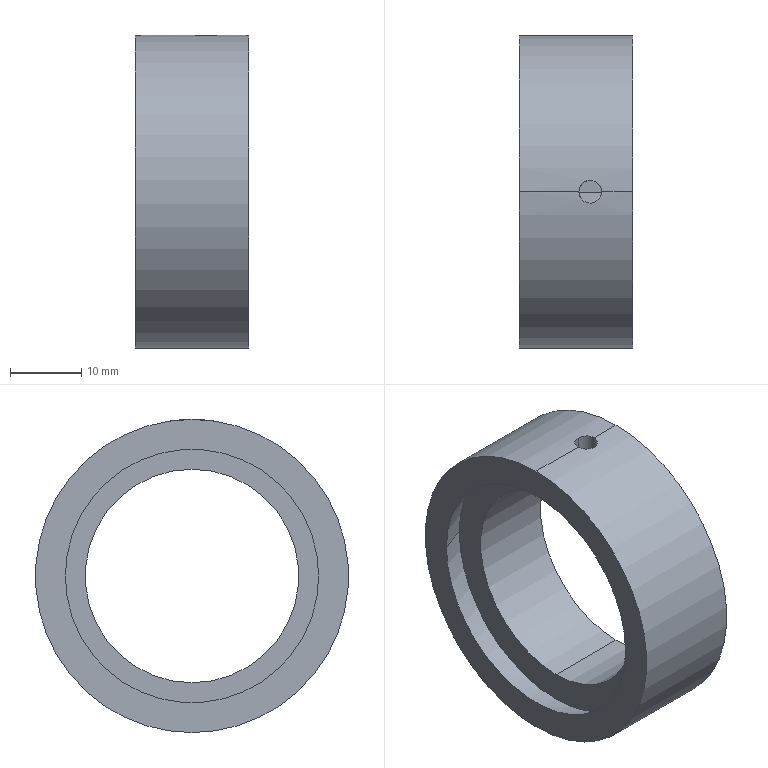Part | SolidWorks | features BaseBody 1 | 1 solid | 11 faces | box 15.9 x 44 x 44 mm | volume 11392 mm3 | cylinder 6 | plane 3 | cone 2 | commonest cylinder face diameters 3.2 x2 30 x2 44 x2
STEP:
#1=CARTESIAN_POINT('',(14.2,63.,20.9));
#2=VERTEX_POINT('',#1);
#3=CARTESIAN_POINT('',(14.2,63.,64.9));
#4=VERTEX_POINT('',#3);
#5=CARTESIAN_POINT('',(14.2,63.,42.9));
#6=DIRECTION('',(1.,0.,0.));
#7=DIRECTION('',(0.,0.,-1.));
#8=AXIS2_PLACEMENT_3D('',#5,#6,#7);
#9=CIRCLE('',#8,22.);
#10=EDGE_CURVE('',#2,#4,#9,.T.);
#11=ORIENTED_EDGE('',*,*,#10,.T.);
#12=CARTESIAN_POINT('',(22.55,63.,64.9));
#13=VERTEX_POINT('',#12);
#14=CARTESIAN_POINT('',(22.15,63.,64.9));
#15=DIRECTION('',(1.,0.,0.));
#16=VECTOR('',#15,1000.);
#17=LINE('',#14,#16);
#18=EDGE_CURVE('',#4,#13,#17,.T.);
#19=ORIENTED_EDGE('',*,*,#18,.T.);
#20=CARTESIAN_POINT('',(24.15,64.6,64.842));
#21=VERTEX_POINT('',#20);
#22=CARTESIAN_POINT('',(22.55,63.,64.9));
#23=CARTESIAN_POINT('',(22.55,63.106,64.9));
#24=CARTESIAN_POINT('',(22.56,63.21,64.899));
#25=CARTESIAN_POINT('',(22.601,63.414,64.896));
#26=CARTESIAN_POINT('',(22.632,63.516,64.894));
#27=CARTESIAN_POINT('',(22.712,63.71,64.889));
#28=CARTESIAN_POINT('',(22.761,63.802,64.886));
#29=CARTESIAN_POINT('',(22.878,63.976,64.879));
#30=CARTESIAN_POINT('',(22.945,64.058,64.875));
#31=CARTESIAN_POINT('',(23.167,64.279,64.863));
#32=CARTESIAN_POINT('',(23.345,64.399,64.856));
#33=CARTESIAN_POINT('',(23.73,64.558,64.845));
#34=CARTESIAN_POINT('',(23.941,64.6,64.842));
#35=CARTESIAN_POINT('',(24.15,64.6,64.842));
#36=B_SPLINE_CURVE_WITH_KNOTS('',3,(#22,#23,#24,#25,#26,#27,#28,#29,#30,#31,#32,#33,#34,#35),.UNSPECIFIED.,.F.,.F.,(4,2,2,2,2,2,4),(0.,0.0003128,0.0006256,0.0009385,0.001251,0.001877,0.002503),.UNSPECIFIED.);
#37=EDGE_CURVE('',#13,#21,#36,.T.);
#38=ORIENTED_EDGE('',*,*,#37,.T.);
#39=CARTESIAN_POINT('',(25.75,63.,64.9));
#40=VERTEX_POINT('',#39);
#41=CARTESIAN_POINT('',(24.15,64.6,64.842));
#42=CARTESIAN_POINT('',(24.254,64.6,64.842));
#43=CARTESIAN_POINT('',(24.36,64.59,64.843));
#44=CARTESIAN_POINT('',(24.566,64.549,64.845));
#45=CARTESIAN_POINT('',(24.665,64.518,64.848));
#46=CARTESIAN_POINT('',(24.859,64.438,64.853));
#47=CARTESIAN_POINT('',(24.953,64.388,64.856));
#48=CARTESIAN_POINT('',(25.126,64.272,64.863));
#49=CARTESIAN_POINT('',(25.207,64.206,64.867));
#50=CARTESIAN_POINT('',(25.356,64.057,64.875));
#51=CARTESIAN_POINT('',(25.422,63.976,64.879));
#52=CARTESIAN_POINT('',(25.538,63.803,64.886));
#53=CARTESIAN_POINT('',(25.588,63.709,64.889));
#54=CARTESIAN_POINT('',(25.668,63.515,64.894));
#55=CARTESIAN_POINT('',(25.699,63.416,64.896));
#56=CARTESIAN_POINT('',(25.74,63.21,64.899));
#57=CARTESIAN_POINT('',(25.75,63.104,64.9));
#58=CARTESIAN_POINT('',(25.75,63.,64.9));
#59=B_SPLINE_CURVE_WITH_KNOTS('',3,(#41,#42,#43,#44,#45,#46,#47,#48,#49,#50,#51,#52,#53,#54,#55,#56,#57,#58),.UNSPECIFIED.,.F.,.F.,(4,2,2,2,2,2,2,2,4),(0.002503,0.002815,0.003128,0.003441,0.003753,0.004066,0.004379,0.004691,0.005004),.UNSPECIFIED.);
#60=EDGE_CURVE('',#21,#40,#59,.T.);
#61=ORIENTED_EDGE('',*,*,#60,.T.);
#62=CARTESIAN_POINT('',(30.1,63.,64.9));
#63=VERTEX_POINT('',#62);
#64=CARTESIAN_POINT('',(22.15,63.,64.9));
#65=DIRECTION('',(1.,0.,0.));
#66=VECTOR('',#65,1000.);
#67=LINE('',#64,#66);
#68=EDGE_CURVE('',#40,#63,#67,.T.);
#69=ORIENTED_EDGE('',*,*,#68,.T.);
#70=CARTESIAN_POINT('',(30.1,63.,20.9));
#71=VERTEX_POINT('',#70);
#72=CARTESIAN_POINT('',(30.1,63.,42.9));
#73=DIRECTION('',(-1.,0.,0.));
#74=DIRECTION('',(0.,0.,-1.));
#75=AXIS2_PLACEMENT_3D('',#72,#73,#74);
#76=CIRCLE('',#75,22.);
#77=EDGE_CURVE('',#63,#71,#76,.T.);
#78=ORIENTED_EDGE('',*,*,#77,.T.);
#79=CARTESIAN_POINT('',(22.15,63.,20.9));
#80=DIRECTION('',(1.,0.,0.));
#81=VECTOR('',#80,1000.);
#82=LINE('',#79,#81);
#83=EDGE_CURVE('',#2,#71,#82,.T.);
#84=ORIENTED_EDGE('',*,*,#83,.F.);
#85=EDGE_LOOP('',(#11,#19,#38,#61,#69,#78,#84));
#86=FACE_OUTER_BOUND('',#85,.T.);
#87=CARTESIAN_POINT('',(22.15,63.,42.9));
#88=DIRECTION('',(1.,0.,0.));
#89=DIRECTION('',(0.,0.,-1.));
#90=AXIS2_PLACEMENT_3D('',#87,#88,#89);
#91=CYLINDRICAL_SURFACE('',#90,22.);
#92=ADVANCED_FACE('',(#86),#91,.T.);
#93=CARTESIAN_POINT('',(24.15,61.4,64.842));
#94=VERTEX_POINT('',#93);
#95=CARTESIAN_POINT('',(24.15,61.4,64.842));
#96=CARTESIAN_POINT('',(24.044,61.4,64.842));
#97=CARTESIAN_POINT('',(23.94,61.41,64.843));
#98=CARTESIAN_POINT('',(23.736,61.451,64.845));
#99=CARTESIAN_POINT('',(23.634,61.482,64.848));
#100=CARTESIAN_POINT('',(23.441,61.562,64.853));
#101=CARTESIAN_POINT('',(23.349,61.611,64.856));
#102=CARTESIAN_POINT('',(23.175,61.727,64.863));
#103=CARTESIAN_POINT('',(23.093,61.795,64.867));
#104=CARTESIAN_POINT('',(22.871,62.016,64.878));
#105=CARTESIAN_POINT('',(22.752,62.194,64.886));
#106=CARTESIAN_POINT('',(22.592,62.579,64.897));
#107=CARTESIAN_POINT('',(22.55,62.789,64.9));
#108=CARTESIAN_POINT('',(22.55,63.,64.9));
#109=B_SPLINE_CURVE_WITH_KNOTS('',3,(#95,#96,#97,#98,#99,#100,#101,#102,#103,#104,#105,#106,#107,#108),.UNSPECIFIED.,.F.,.F.,(4,2,2,2,2,2,4),(0.007507,0.007819,0.008132,0.008444,0.008757,0.009382,0.01001),.UNSPECIFIED.);
#110=EDGE_CURVE('',#94,#13,#109,.T.);
#111=ORIENTED_EDGE('',*,*,#110,.F.);
#112=CARTESIAN_POINT('',(24.15,61.4,57.814));
#113=VERTEX_POINT('',#112);
#114=CARTESIAN_POINT('',(24.15,61.4,60.875));
#115=DIRECTION('',(0.,0.,-1.));
#116=VECTOR('',#115,1000.);
#117=LINE('',#114,#116);
#118=EDGE_CURVE('',#94,#113,#117,.T.);
#119=ORIENTED_EDGE('',*,*,#118,.T.);
#120=CARTESIAN_POINT('',(22.55,63.,57.9));
#121=VERTEX_POINT('',#120);
#122=CARTESIAN_POINT('',(22.55,63.,57.9));
#123=CARTESIAN_POINT('',(22.55,62.894,57.9));
#124=CARTESIAN_POINT('',(22.56,62.79,57.899));
#125=CARTESIAN_POINT('',(22.601,62.585,57.895));
#126=CARTESIAN_POINT('',(22.632,62.484,57.891));
#127=CARTESIAN_POINT('',(22.712,62.29,57.884));
#128=CARTESIAN_POINT('',(22.762,62.198,57.879));
#129=CARTESIAN_POINT('',(22.878,62.024,57.868));
#130=CARTESIAN_POINT('',(22.945,61.942,57.863));
#131=CARTESIAN_POINT('',(23.167,61.721,57.846));
#132=CARTESIAN_POINT('',(23.345,61.602,57.835));
#133=CARTESIAN_POINT('',(23.73,61.442,57.819));
#134=CARTESIAN_POINT('',(23.941,61.4,57.814));
#135=CARTESIAN_POINT('',(24.15,61.4,57.814));
#136=B_SPLINE_CURVE_WITH_KNOTS('',3,(#122,#123,#124,#125,#126,#127,#128,#129,#130,#131,#132,#133,#134,#135),.UNSPECIFIED.,.F.,.F.,(4,2,2,2,2,2,4),(0.002501,0.002814,0.003127,0.00344,0.003753,0.004379,0.005005),.UNSPECIFIED.);
#137=EDGE_CURVE('',#121,#113,#136,.T.);
#138=ORIENTED_EDGE('',*,*,#137,.F.);
#139=CARTESIAN_POINT('',(24.15,64.6,57.814));
#140=VERTEX_POINT('',#139);
#141=CARTESIAN_POINT('',(24.15,64.6,57.814));
#142=CARTESIAN_POINT('',(24.044,64.6,57.814));
#143=CARTESIAN_POINT('',(23.94,64.59,57.816));
#144=CARTESIAN_POINT('',(23.736,64.549,57.82));
#145=CARTESIAN_POINT('',(23.634,64.518,57.823));
#146=CARTESIAN_POINT('',(23.441,64.438,57.831));
#147=CARTESIAN_POINT('',(23.349,64.389,57.836));
#148=CARTESIAN_POINT('',(23.175,64.273,57.846));
#149=CARTESIAN_POINT('',(23.093,64.205,57.852));
#150=CARTESIAN_POINT('',(22.872,63.984,57.868));
#151=CARTESIAN_POINT('',(22.752,63.806,57.88));
#152=CARTESIAN_POINT('',(22.593,63.422,57.895));
#153=CARTESIAN_POINT('',(22.55,63.211,57.9));
#154=CARTESIAN_POINT('',(22.55,63.,57.9));
#155=B_SPLINE_CURVE_WITH_KNOTS('',3,(#141,#142,#143,#144,#145,#146,#147,#148,#149,#150,#151,#152,#153,#154),.UNSPECIFIED.,.F.,.F.,(4,2,2,2,2,2,4),(0.,0.0003127,0.0006253,0.000938,0.001251,0.001876,0.002501),.UNSPECIFIED.);
#156=EDGE_CURVE('',#140,#121,#155,.T.);
#157=ORIENTED_EDGE('',*,*,#156,.F.);
#158=CARTESIAN_POINT('',(24.15,64.6,60.875));
#159=DIRECTION('',(0.,0.,-1.));
#160=VECTOR('',#159,1000.);
#161=LINE('',#158,#160);
#162=EDGE_CURVE('',#21,#140,#161,.T.);
#163=ORIENTED_EDGE('',*,*,#162,.F.);
#164=ORIENTED_EDGE('',*,*,#37,.F.);
#165=EDGE_LOOP('',(#111,#119,#138,#157,#163,#164));
#166=FACE_OUTER_BOUND('',#165,.T.);
#167=CARTESIAN_POINT('',(24.15,63.,60.875));
#168=DIRECTION('',(0.,0.,-1.));
#169=DIRECTION('',(0.,1.,0.));
#170=AXIS2_PLACEMENT_3D('',#167,#168,#169);
#171=CYLINDRICAL_SURFACE('',#170,1.6);
#172=ADVANCED_FACE('',(#166),#171,.F.);
#173=CARTESIAN_POINT('',(14.2,45.2,42.9));
#174=VERTEX_POINT('',#173);
#175=CARTESIAN_POINT('',(14.2,80.8,42.9));
#176=VERTEX_POINT('',#175);
#177=CARTESIAN_POINT('',(14.2,63.,42.9));
#178=DIRECTION('',(1.,0.,0.));
#179=DIRECTION('',(0.,1.,0.));
#180=AXIS2_PLACEMENT_3D('',#177,#178,#179);
#181=CIRCLE('',#180,17.8);
#182=EDGE_CURVE('',#174,#176,#181,.T.);
#183=ORIENTED_EDGE('',*,*,#182,.F.);
#184=CARTESIAN_POINT('',(18.2,43.744,42.9));
#185=VERTEX_POINT('',#184);
#186=CARTESIAN_POINT('',(14.2,45.2,42.9));
#187=DIRECTION('',(0.9397,-0.342,0.));
#188=VECTOR('',#187,1000.);
#189=LINE('',#186,#188);
#190=EDGE_CURVE('',#174,#185,#189,.T.);
#191=ORIENTED_EDGE('',*,*,#190,.T.);
#192=CARTESIAN_POINT('',(18.2,82.256,42.9));
#193=VERTEX_POINT('',#192);
#194=CARTESIAN_POINT('',(18.2,63.,42.9));
#195=DIRECTION('',(1.,0.,0.));
#196=DIRECTION('',(0.,1.,0.));
#197=AXIS2_PLACEMENT_3D('',#194,#195,#196);
#198=CIRCLE('',#197,19.256);
#199=EDGE_CURVE('',#185,#193,#198,.T.);
#200=ORIENTED_EDGE('',*,*,#199,.T.);
#201=CARTESIAN_POINT('',(14.2,80.8,42.9));
#202=DIRECTION('',(0.9397,0.342,0.));
#203=VECTOR('',#202,1000.);
#204=LINE('',#201,#203);
#205=EDGE_CURVE('',#176,#193,#204,.T.);
#206=ORIENTED_EDGE('',*,*,#205,.F.);
#207=EDGE_LOOP('',(#183,#191,#200,#206));
#208=FACE_OUTER_BOUND('',#207,.T.);
#209=CARTESIAN_POINT('',(14.2,63.,42.9));
#210=DIRECTION('',(1.,0.,0.));
#211=DIRECTION('',(0.,1.,0.));
#212=AXIS2_PLACEMENT_3D('',#209,#210,#211);
#213=CONICAL_SURFACE('',#212,17.8,0.3491);
#214=ADVANCED_FACE('',(#208),#213,.F.);
#215=CARTESIAN_POINT('',(18.2,63.,27.9));
#216=VERTEX_POINT('',#215);
#217=CARTESIAN_POINT('',(18.2,63.,57.9));
#218=VERTEX_POINT('',#217);
#219=CARTESIAN_POINT('',(18.2,63.,42.9));
#220=DIRECTION('',(-1.,0.,0.));
#221=DIRECTION('',(0.,0.,-1.));
#222=AXIS2_PLACEMENT_3D('',#219,#220,#221);
#223=CIRCLE('',#222,15.);
#224=EDGE_CURVE('',#216,#218,#223,.T.);
#225=ORIENTED_EDGE('',*,*,#224,.T.);
#226=CARTESIAN_POINT('',(18.2,63.,57.9));
#227=DIRECTION('',(1.,0.,0.));
#228=VECTOR('',#227,1000.);
#229=LINE('',#226,#228);
#230=EDGE_CURVE('',#218,#121,#229,.T.);
#231=ORIENTED_EDGE('',*,*,#230,.T.);
#232=ORIENTED_EDGE('',*,*,#137,.T.);
#233=CARTESIAN_POINT('',(25.75,63.,57.9));
#234=VERTEX_POINT('',#233);
#235=CARTESIAN_POINT('',(24.15,61.4,57.814));
#236=CARTESIAN_POINT('',(24.254,61.4,57.814));
#237=CARTESIAN_POINT('',(24.36,61.41,57.816));
#238=CARTESIAN_POINT('',(24.566,61.451,57.82));
#239=CARTESIAN_POINT('',(24.665,61.482,57.823));
#240=CARTESIAN_POINT('',(24.859,61.562,57.831));
#241=CARTESIAN_POINT('',(24.952,61.612,57.836));
#242=CARTESIAN_POINT('',(25.126,61.728,57.846));
#243=CARTESIAN_POINT('',(25.206,61.794,57.852));
#244=CARTESIAN_POINT('',(25.356,61.943,57.863));
#245=CARTESIAN_POINT('',(25.422,62.024,57.868));
#246=CARTESIAN_POINT('',(25.538,62.197,57.879));
#247=CARTESIAN_POINT('',(25.588,62.29,57.884));
#248=CARTESIAN_POINT('',(25.708,62.581,57.895));
#249=CARTESIAN_POINT('',(25.75,62.789,57.9));
#250=CARTESIAN_POINT('',(25.75,63.,57.9));
#251=B_SPLINE_CURVE_WITH_KNOTS('',3,(#235,#236,#237,#238,#239,#240,#241,#242,#243,#244,#245,#246,#247,#248,#249,#250),.UNSPECIFIED.,.F.,.F.,(4,2,2,2,2,2,2,4),(0.005005,0.005317,0.00563,0.005943,0.006255,0.006568,0.006881,0.007506),.UNSPECIFIED.);
#252=EDGE_CURVE('',#113,#234,#251,.T.);
#253=ORIENTED_EDGE('',*,*,#252,.T.);
#254=CARTESIAN_POINT('',(30.1,63.,57.9));
#255=VERTEX_POINT('',#254);
#256=CARTESIAN_POINT('',(18.2,63.,57.9));
#257=DIRECTION('',(1.,0.,0.));
#258=VECTOR('',#257,1000.);
#259=LINE('',#256,#258);
#260=EDGE_CURVE('',#234,#255,#259,.T.);
#261=ORIENTED_EDGE('',*,*,#260,.T.);
#262=CARTESIAN_POINT('',(30.1,63.,27.9));
#263=VERTEX_POINT('',#262);
#264=CARTESIAN_POINT('',(30.1,63.,42.9));
#265=DIRECTION('',(-1.,0.,0.));
#266=DIRECTION('',(0.,0.,-1.));
#267=AXIS2_PLACEMENT_3D('',#264,#265,#266);
#268=CIRCLE('',#267,15.);
#269=EDGE_CURVE('',#263,#255,#268,.T.);
#270=ORIENTED_EDGE('',*,*,#269,.F.);
#271=CARTESIAN_POINT('',(18.2,63.,27.9));
#272=DIRECTION('',(1.,0.,0.));
#273=VECTOR('',#272,1000.);
#274=LINE('',#271,#273);
#275=EDGE_CURVE('',#216,#263,#274,.T.);
#276=ORIENTED_EDGE('',*,*,#275,.F.);
#277=EDGE_LOOP('',(#225,#231,#232,#253,#261,#270,#276));
#278=FACE_OUTER_BOUND('',#277,.T.);
#279=CARTESIAN_POINT('',(18.2,63.,42.9));
#280=DIRECTION('',(1.,0.,0.));
#281=DIRECTION('',(0.,0.,-1.));
#282=AXIS2_PLACEMENT_3D('',#279,#280,#281);
#283=CYLINDRICAL_SURFACE('',#282,15.);
#284=ADVANCED_FACE('',(#278),#283,.F.);
#285=ORIENTED_EDGE('',*,*,#18,.F.);
#286=CARTESIAN_POINT('',(14.2,63.,42.9));
#287=DIRECTION('',(1.,0.,0.));
#288=DIRECTION('',(0.,0.,-1.));
#289=AXIS2_PLACEMENT_3D('',#286,#287,#288);
#290=CIRCLE('',#289,22.);
#291=EDGE_CURVE('',#4,#2,#290,.T.);
#292=ORIENTED_EDGE('',*,*,#291,.T.);
#293=ORIENTED_EDGE('',*,*,#83,.T.);
#294=CARTESIAN_POINT('',(30.1,63.,42.9));
#295=DIRECTION('',(-1.,0.,0.));
#296=DIRECTION('',(0.,0.,-1.));
#297=AXIS2_PLACEMENT_3D('',#294,#295,#296);
#298=CIRCLE('',#297,22.);
#299=EDGE_CURVE('',#71,#63,#298,.T.);
#300=ORIENTED_EDGE('',*,*,#299,.T.);
#301=ORIENTED_EDGE('',*,*,#68,.F.);
#302=CARTESIAN_POINT('',(25.75,63.,64.9));
#303=CARTESIAN_POINT('',(25.75,62.791,64.9));
#304=CARTESIAN_POINT('',(25.708,62.58,64.897));
#305=CARTESIAN_POINT('',(25.548,62.195,64.886));
#306=CARTESIAN_POINT('',(25.429,62.017,64.879));
#307=CARTESIAN_POINT('',(25.208,61.795,64.867));
#308=CARTESIAN_POINT('',(25.126,61.728,64.863));
#309=CARTESIAN_POINT('',(24.952,61.611,64.856));
#310=CARTESIAN_POINT('',(24.86,61.562,64.853));
#311=CARTESIAN_POINT('',(24.666,61.482,64.848));
#312=CARTESIAN_POINT('',(24.564,61.451,64.845));
#313=CARTESIAN_POINT('',(24.36,61.41,64.843));
#314=CARTESIAN_POINT('',(24.256,61.4,64.842));
#315=CARTESIAN_POINT('',(24.15,61.4,64.842));
#316=B_SPLINE_CURVE_WITH_KNOTS('',3,(#302,#303,#304,#305,#306,#307,#308,#309,#310,#311,#312,#313,#314,#315),.UNSPECIFIED.,.F.,.F.,(4,2,2,2,2,2,4),(0.005004,0.00563,0.006255,0.006568,0.006881,0.007194,0.007507),.UNSPECIFIED.);
#317=EDGE_CURVE('',#40,#94,#316,.T.);
#318=ORIENTED_EDGE('',*,*,#317,.T.);
#319=ORIENTED_EDGE('',*,*,#110,.T.);
#320=EDGE_LOOP('',(#285,#292,#293,#300,#301,#318,#319));
#321=FACE_OUTER_BOUND('',#320,.T.);
#322=CARTESIAN_POINT('',(22.15,63.,42.9));
#323=DIRECTION('',(1.,0.,0.));
#324=DIRECTION('',(0.,0.,-1.));
#325=AXIS2_PLACEMENT_3D('',#322,#323,#324);
#326=CYLINDRICAL_SURFACE('',#325,22.);
#327=ADVANCED_FACE('',(#321),#326,.T.);
#328=CARTESIAN_POINT('',(14.2,63.,42.9));
#329=DIRECTION('',(1.,0.,0.));
#330=DIRECTION('',(0.,1.,0.));
#331=AXIS2_PLACEMENT_3D('',#328,#329,#330);
#332=CIRCLE('',#331,17.8);
#333=EDGE_CURVE('',#176,#174,#332,.T.);
#334=ORIENTED_EDGE('',*,*,#333,.T.);
#335=ORIENTED_EDGE('',*,*,#182,.T.);
#336=EDGE_LOOP('',(#334,#335));
#337=FACE_BOUND('',#336,.T.);
#338=ORIENTED_EDGE('',*,*,#10,.F.);
#339=ORIENTED_EDGE('',*,*,#291,.F.);
#340=EDGE_LOOP('',(#338,#339));
#341=FACE_OUTER_BOUND('',#340,.T.);
#342=CARTESIAN_POINT('',(14.2,63.,62.8));
#343=DIRECTION('',(-1.,0.,0.));
#344=DIRECTION('',(0.,0.,1.));
#345=AXIS2_PLACEMENT_3D('',#342,#343,#344);
#346=PLANE('',#345);
#347=ADVANCED_FACE('',(#337,#341),#346,.T.);
#348=ORIENTED_EDGE('',*,*,#299,.F.);
#349=ORIENTED_EDGE('',*,*,#77,.F.);
#350=EDGE_LOOP('',(#348,#349));
#351=FACE_OUTER_BOUND('',#350,.T.);
#352=ORIENTED_EDGE('',*,*,#269,.T.);
#353=CARTESIAN_POINT('',(30.1,63.,42.9));
#354=DIRECTION('',(-1.,0.,0.));
#355=DIRECTION('',(0.,0.,-1.));
#356=AXIS2_PLACEMENT_3D('',#353,#354,#355);
#357=CIRCLE('',#356,15.);
#358=EDGE_CURVE('',#255,#263,#357,.T.);
#359=ORIENTED_EDGE('',*,*,#358,.T.);
#360=EDGE_LOOP('',(#352,#359));
#361=FACE_BOUND('',#360,.T.);
#362=CARTESIAN_POINT('',(30.1,63.,61.4));
#363=DIRECTION('',(1.,0.,0.));
#364=DIRECTION('',(0.,0.,-1.));
#365=AXIS2_PLACEMENT_3D('',#362,#363,#364);
#366=PLANE('',#365);
#367=ADVANCED_FACE('',(#351,#361),#366,.T.);
#368=ORIENTED_EDGE('',*,*,#118,.F.);
#369=ORIENTED_EDGE('',*,*,#317,.F.);
#370=ORIENTED_EDGE('',*,*,#60,.F.);
#371=ORIENTED_EDGE('',*,*,#162,.T.);
#372=CARTESIAN_POINT('',(25.75,63.,57.9));
#373=CARTESIAN_POINT('',(25.75,63.106,57.9));
#374=CARTESIAN_POINT('',(25.74,63.21,57.899));
#375=CARTESIAN_POINT('',(25.699,63.414,57.895));
#376=CARTESIAN_POINT('',(25.668,63.516,57.891));
#377=CARTESIAN_POINT('',(25.588,63.709,57.884));
#378=CARTESIAN_POINT('',(25.539,63.801,57.879));
#379=CARTESIAN_POINT('',(25.423,63.975,57.869));
#380=CARTESIAN_POINT('',(25.355,64.057,57.863));
#381=CARTESIAN_POINT('',(25.134,64.278,57.846));
#382=CARTESIAN_POINT('',(24.956,64.398,57.835));
#383=CARTESIAN_POINT('',(24.572,64.557,57.819));
#384=CARTESIAN_POINT('',(24.361,64.6,57.814));
#385=CARTESIAN_POINT('',(24.15,64.6,57.814));
#386=B_SPLINE_CURVE_WITH_KNOTS('',3,(#372,#373,#374,#375,#376,#377,#378,#379,#380,#381,#382,#383,#384,#385),.UNSPECIFIED.,.F.,.F.,(4,2,2,2,2,2,4),(0.007506,0.007819,0.008131,0.008444,0.008757,0.009382,0.01001),.UNSPECIFIED.);
#387=EDGE_CURVE('',#234,#140,#386,.T.);
#388=ORIENTED_EDGE('',*,*,#387,.F.);
#389=ORIENTED_EDGE('',*,*,#252,.F.);
#390=EDGE_LOOP('',(#368,#369,#370,#371,#388,#389));
#391=FACE_OUTER_BOUND('',#390,.T.);
#392=CARTESIAN_POINT('',(24.15,63.,60.875));
#393=DIRECTION('',(0.,0.,-1.));
#394=DIRECTION('',(0.,1.,0.));
#395=AXIS2_PLACEMENT_3D('',#392,#393,#394);
#396=CYLINDRICAL_SURFACE('',#395,1.6);
#397=ADVANCED_FACE('',(#391),#396,.F.);
#398=ORIENTED_EDGE('',*,*,#190,.F.);
#399=ORIENTED_EDGE('',*,*,#333,.F.);
#400=ORIENTED_EDGE('',*,*,#205,.T.);
#401=CARTESIAN_POINT('',(18.2,63.,42.9));
#402=DIRECTION('',(1.,0.,0.));
#403=DIRECTION('',(0.,1.,0.));
#404=AXIS2_PLACEMENT_3D('',#401,#402,#403);
#405=CIRCLE('',#404,19.256);
#406=EDGE_CURVE('',#193,#185,#405,.T.);
#407=ORIENTED_EDGE('',*,*,#406,.T.);
#408=EDGE_LOOP('',(#398,#399,#400,#407));
#409=FACE_OUTER_BOUND('',#408,.T.);
#410=CARTESIAN_POINT('',(14.2,63.,42.9));
#411=DIRECTION('',(1.,0.,0.));
#412=DIRECTION('',(0.,1.,0.));
#413=AXIS2_PLACEMENT_3D('',#410,#411,#412);
#414=CONICAL_SURFACE('',#413,17.8,0.3491);
#415=ADVANCED_FACE('',(#409),#414,.F.);
#416=ORIENTED_EDGE('',*,*,#230,.F.);
#417=CARTESIAN_POINT('',(18.2,63.,42.9));
#418=DIRECTION('',(-1.,0.,0.));
#419=DIRECTION('',(0.,0.,-1.));
#420=AXIS2_PLACEMENT_3D('',#417,#418,#419);
#421=CIRCLE('',#420,15.);
#422=EDGE_CURVE('',#218,#216,#421,.T.);
#423=ORIENTED_EDGE('',*,*,#422,.T.);
#424=ORIENTED_EDGE('',*,*,#275,.T.);
#425=ORIENTED_EDGE('',*,*,#358,.F.);
#426=ORIENTED_EDGE('',*,*,#260,.F.);
#427=ORIENTED_EDGE('',*,*,#387,.T.);
#428=ORIENTED_EDGE('',*,*,#156,.T.);
#429=EDGE_LOOP('',(#416,#423,#424,#425,#426,#427,#428));
#430=FACE_OUTER_BOUND('',#429,.T.);
#431=CARTESIAN_POINT('',(18.2,63.,42.9));
#432=DIRECTION('',(1.,0.,0.));
#433=DIRECTION('',(0.,0.,-1.));
#434=AXIS2_PLACEMENT_3D('',#431,#432,#433);
#435=CYLINDRICAL_SURFACE('',#434,15.);
#436=ADVANCED_FACE('',(#430),#435,.F.);
#437=ORIENTED_EDGE('',*,*,#224,.F.);
#438=ORIENTED_EDGE('',*,*,#422,.F.);
#439=EDGE_LOOP('',(#437,#438));
#440=FACE_BOUND('',#439,.T.);
#441=ORIENTED_EDGE('',*,*,#406,.F.);
#442=ORIENTED_EDGE('',*,*,#199,.F.);
#443=EDGE_LOOP('',(#441,#442));
#444=FACE_OUTER_BOUND('',#443,.T.);
#445=CARTESIAN_POINT('',(18.2,63.,60.028));
#446=DIRECTION('',(-1.,0.,0.));
#447=DIRECTION('',(0.,0.,1.));
#448=AXIS2_PLACEMENT_3D('',#445,#446,#447);
#449=PLANE('',#448);
#450=ADVANCED_FACE('',(#440,#444),#449,.T.);
#451=CLOSED_SHELL('',(#92,#172,#214,#284,#327,#347,#367,#397,#415,#436,#450));
#452=MANIFOLD_SOLID_BREP('',#451);
#453=CARTESIAN_POINT('',(0.,0.,0.));
#454=DIRECTION('',(0.,0.,1.));
#455=DIRECTION('',(1.,0.,0.));
#456=AXIS2_PLACEMENT_3D('',#453,#454,#455);
#457=(LENGTH_UNIT()NAMED_UNIT(*)SI_UNIT(.MILLI.,.METRE.));
#458=UNCERTAINTY_MEASURE_WITH_UNIT(LENGTH_MEASURE(0.00001),#457,'','');
#459=(NAMED_UNIT(*)PLANE_ANGLE_UNIT()SI_UNIT($,.RADIAN.));
#460=(NAMED_UNIT(*)SI_UNIT($,.STERADIAN.)SOLID_ANGLE_UNIT());
#461=(GEOMETRIC_REPRESENTATION_CONTEXT(3)GLOBAL_UNCERTAINTY_ASSIGNED_CONTEXT((#458))GLOBAL_UNIT_ASSIGNED_CONTEXT((#457,#459,#460))REPRESENTATION_CONTEXT('',''));
#462=ADVANCED_BREP_SHAPE_REPRESENTATION('',(#452,#456),#461);